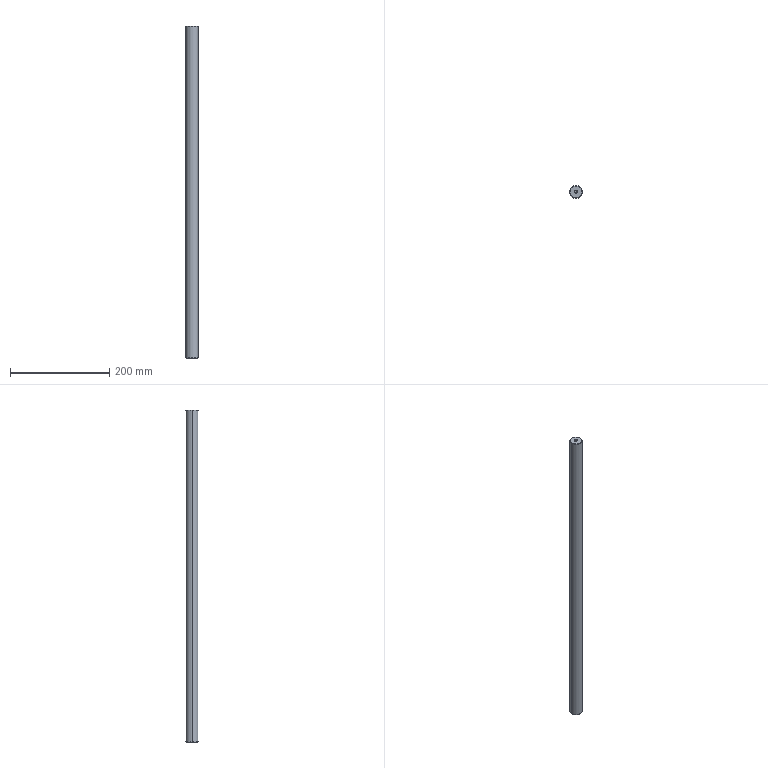Part | STEP file | 1 solid | 20 faces | box 25 x 25 x 670 mm | volume 328039 mm3 | cone 12 | cylinder 6 | plane 2 | commonest cylinder face diameters 5 x4 25 x2
STEP:
#1=CARTESIAN_POINT('',(0.,0.,0.));
#2=DIRECTION('',(0.,0.,1.));
#3=DIRECTION('',(1.,0.,0.));
#4=AXIS2_PLACEMENT_3D('',#1,#2,#3);
#5=CARTESIAN_POINT('',(488.025,0.,665.));
#6=VERTEX_POINT('',#5);
#7=CARTESIAN_POINT('',(481.975,0.,665.));
#8=VERTEX_POINT('',#7);
#9=CARTESIAN_POINT('',(485.,0.,665.));
#10=DIRECTION('',(0.,0.,1.));
#11=DIRECTION('',(1.,0.,0.));
#12=AXIS2_PLACEMENT_3D('',#9,#10,#11);
#13=CIRCLE('',#12,3.025);
#14=CARTESIAN_POINT('',(485.,0.,665.));
#15=DIRECTION('',(0.,0.,1.));
#16=DIRECTION('',(1.,0.,0.));
#17=AXIS2_PLACEMENT_3D('',#14,#15,#16);
#18=CONICAL_SURFACE('',#17,3.025,0.7854);
#19=CARTESIAN_POINT('',(0.,0.));
#20=DIRECTION('',(1.,0.));
#21=VECTOR('',#20,1.);
#22=LINE('',#19,#21);
#23=(GEOMETRIC_REPRESENTATION_CONTEXT(2)PARAMETRIC_REPRESENTATION_CONTEXT()REPRESENTATION_CONTEXT('',''));
#24=DEFINITIONAL_REPRESENTATION('',(#22),#23);
#25=PCURVE('',#18,#24);
#26=CARTESIAN_POINT('',(485.,0.,665.));
#27=DIRECTION('',(0.,0.,1.));
#28=DIRECTION('',(0.,-1.,0.));
#29=AXIS2_PLACEMENT_3D('',#26,#27,#28);
#30=PLANE('',#29);
#31=CARTESIAN_POINT('',(0.,0.));
#32=DIRECTION('',(0.,1.));
#33=AXIS2_PLACEMENT_2D('',#31,#32);
#34=CIRCLE('',#33,3.025);
#35=(GEOMETRIC_REPRESENTATION_CONTEXT(2)PARAMETRIC_REPRESENTATION_CONTEXT()REPRESENTATION_CONTEXT('',''));
#36=DEFINITIONAL_REPRESENTATION('',(#34),#35);
#37=PCURVE('',#30,#36);
#38=SURFACE_CURVE('',#13,(#25,#37),.PCURVE_S1.);
#39=EDGE_CURVE('',#6,#8,#38,.T.);
#40=ORIENTED_EDGE('',*,*,#39,.F.);
#41=CARTESIAN_POINT('',(487.5,0.,664.475));
#42=VERTEX_POINT('',#41);
#43=CARTESIAN_POINT('',(488.025,0.,665.));
#44=DIRECTION('',(0.7071,0.,0.7071));
#45=VECTOR('',#44,1.);
#46=LINE('',#43,#45);
#47=CARTESIAN_POINT('',(0.,0.));
#48=DIRECTION('',(0.,1.));
#49=VECTOR('',#48,1.);
#50=LINE('',#47,#49);
#51=(GEOMETRIC_REPRESENTATION_CONTEXT(2)PARAMETRIC_REPRESENTATION_CONTEXT()REPRESENTATION_CONTEXT('',''));
#52=DEFINITIONAL_REPRESENTATION('',(#50),#51);
#53=PCURVE('',#18,#52);
#54=CARTESIAN_POINT('',(485.,0.,665.));
#55=DIRECTION('',(0.,0.,1.));
#56=DIRECTION('',(1.,0.,0.));
#57=AXIS2_PLACEMENT_3D('',#54,#55,#56);
#58=CONICAL_SURFACE('',#57,3.025,0.7854);
#59=CARTESIAN_POINT('',(6.283,0.));
#60=DIRECTION('',(0.,1.));
#61=VECTOR('',#60,1.);
#62=LINE('',#59,#61);
#63=(GEOMETRIC_REPRESENTATION_CONTEXT(2)PARAMETRIC_REPRESENTATION_CONTEXT()REPRESENTATION_CONTEXT('',''));
#64=DEFINITIONAL_REPRESENTATION('',(#62),#63);
#65=PCURVE('',#58,#64);
#66=SURFACE_CURVE('',#46,(#53,#65),.PCURVE_S1.);
#67=EDGE_CURVE('',#42,#6,#66,.T.);
#68=ORIENTED_EDGE('',*,*,#67,.F.);
#69=CARTESIAN_POINT('',(482.5,0.,664.475));
#70=VERTEX_POINT('',#69);
#71=CARTESIAN_POINT('',(485.,0.,664.475));
#72=DIRECTION('',(0.,0.,1.));
#73=DIRECTION('',(1.,0.,0.));
#74=AXIS2_PLACEMENT_3D('',#71,#72,#73);
#75=CIRCLE('',#74,2.5);
#76=CARTESIAN_POINT('',(0.,-0.525));
#77=DIRECTION('',(1.,0.));
#78=VECTOR('',#77,1.);
#79=LINE('',#76,#78);
#80=(GEOMETRIC_REPRESENTATION_CONTEXT(2)PARAMETRIC_REPRESENTATION_CONTEXT()REPRESENTATION_CONTEXT('',''));
#81=DEFINITIONAL_REPRESENTATION('',(#79),#80);
#82=PCURVE('',#18,#81);
#83=CARTESIAN_POINT('',(485.,0.,665.));
#84=DIRECTION('',(0.,0.,1.));
#85=DIRECTION('',(1.,0.,0.));
#86=AXIS2_PLACEMENT_3D('',#83,#84,#85);
#87=CYLINDRICAL_SURFACE('',#86,2.5);
#88=CARTESIAN_POINT('',(0.,-0.525));
#89=DIRECTION('',(1.,0.));
#90=VECTOR('',#89,1.);
#91=LINE('',#88,#90);
#92=(GEOMETRIC_REPRESENTATION_CONTEXT(2)PARAMETRIC_REPRESENTATION_CONTEXT()REPRESENTATION_CONTEXT('',''));
#93=DEFINITIONAL_REPRESENTATION('',(#91),#92);
#94=PCURVE('',#87,#93);
#95=SURFACE_CURVE('',#75,(#82,#94),.PCURVE_S1.);
#96=EDGE_CURVE('',#42,#70,#95,.T.);
#97=ORIENTED_EDGE('',*,*,#96,.T.);
#98=CARTESIAN_POINT('',(481.975,0.,665.));
#99=DIRECTION('',(-0.7071,0.,0.7071));
#100=VECTOR('',#99,1.);
#101=LINE('',#98,#100);
#102=CARTESIAN_POINT('',(3.142,0.));
#103=DIRECTION('',(0.,1.));
#104=VECTOR('',#103,1.);
#105=LINE('',#102,#104);
#106=(GEOMETRIC_REPRESENTATION_CONTEXT(2)PARAMETRIC_REPRESENTATION_CONTEXT()REPRESENTATION_CONTEXT('',''));
#107=DEFINITIONAL_REPRESENTATION('',(#105),#106);
#108=PCURVE('',#18,#107);
#109=CARTESIAN_POINT('',(3.142,0.));
#110=DIRECTION('',(0.,1.));
#111=VECTOR('',#110,1.);
#112=LINE('',#109,#111);
#113=(GEOMETRIC_REPRESENTATION_CONTEXT(2)PARAMETRIC_REPRESENTATION_CONTEXT()REPRESENTATION_CONTEXT('',''));
#114=DEFINITIONAL_REPRESENTATION('',(#112),#113);
#115=PCURVE('',#58,#114);
#116=SURFACE_CURVE('',#101,(#108,#115),.PCURVE_S1.);
#117=EDGE_CURVE('',#70,#8,#116,.T.);
#118=ORIENTED_EDGE('',*,*,#117,.T.);
#119=EDGE_LOOP('',(#40,#68,#97,#118));
#120=FACE_BOUND('',#119,.F.);
#121=ADVANCED_FACE('',(#120),#18,.F.);
#122=ORIENTED_EDGE('',*,*,#96,.F.);
#123=CARTESIAN_POINT('',(487.5,0.,650.));
#124=VERTEX_POINT('',#123);
#125=CARTESIAN_POINT('',(487.5,0.,665.));
#126=DIRECTION('',(0.,0.,1.));
#127=VECTOR('',#126,1.);
#128=LINE('',#125,#127);
#129=CARTESIAN_POINT('',(0.,0.));
#130=DIRECTION('',(0.,1.));
#131=VECTOR('',#130,1.);
#132=LINE('',#129,#131);
#133=(GEOMETRIC_REPRESENTATION_CONTEXT(2)PARAMETRIC_REPRESENTATION_CONTEXT()REPRESENTATION_CONTEXT('',''));
#134=DEFINITIONAL_REPRESENTATION('',(#132),#133);
#135=PCURVE('',#87,#134);
#136=CARTESIAN_POINT('',(485.,0.,665.));
#137=DIRECTION('',(0.,0.,1.));
#138=DIRECTION('',(1.,0.,0.));
#139=AXIS2_PLACEMENT_3D('',#136,#137,#138);
#140=CYLINDRICAL_SURFACE('',#139,2.5);
#141=CARTESIAN_POINT('',(6.283,0.));
#142=DIRECTION('',(0.,1.));
#143=VECTOR('',#142,1.);
#144=LINE('',#141,#143);
#145=(GEOMETRIC_REPRESENTATION_CONTEXT(2)PARAMETRIC_REPRESENTATION_CONTEXT()REPRESENTATION_CONTEXT('',''));
#146=DEFINITIONAL_REPRESENTATION('',(#144),#145);
#147=PCURVE('',#140,#146);
#148=SURFACE_CURVE('',#128,(#135,#147),.PCURVE_S1.);
#149=EDGE_CURVE('',#124,#42,#148,.T.);
#150=ORIENTED_EDGE('',*,*,#149,.F.);
#151=CARTESIAN_POINT('',(482.5,0.,650.));
#152=VERTEX_POINT('',#151);
#153=CARTESIAN_POINT('',(485.,0.,650.));
#154=DIRECTION('',(0.,0.,1.));
#155=DIRECTION('',(1.,0.,0.));
#156=AXIS2_PLACEMENT_3D('',#153,#154,#155);
#157=CIRCLE('',#156,2.5);
#158=CARTESIAN_POINT('',(0.,-15.));
#159=DIRECTION('',(1.,0.));
#160=VECTOR('',#159,1.);
#161=LINE('',#158,#160);
#162=(GEOMETRIC_REPRESENTATION_CONTEXT(2)PARAMETRIC_REPRESENTATION_CONTEXT()REPRESENTATION_CONTEXT('',''));
#163=DEFINITIONAL_REPRESENTATION('',(#161),#162);
#164=PCURVE('',#87,#163);
#165=CARTESIAN_POINT('',(485.,0.,650.));
#166=DIRECTION('',(0.,0.,1.));
#167=DIRECTION('',(1.,0.,0.));
#168=AXIS2_PLACEMENT_3D('',#165,#166,#167);
#169=CONICAL_SURFACE('',#168,2.5,1.03);
#170=CARTESIAN_POINT('',(0.,0.));
#171=DIRECTION('',(1.,0.));
#172=VECTOR('',#171,1.);
#173=LINE('',#170,#172);
#174=(GEOMETRIC_REPRESENTATION_CONTEXT(2)PARAMETRIC_REPRESENTATION_CONTEXT()REPRESENTATION_CONTEXT('',''));
#175=DEFINITIONAL_REPRESENTATION('',(#173),#174);
#176=PCURVE('',#169,#175);
#177=SURFACE_CURVE('',#157,(#164,#176),.PCURVE_S1.);
#178=EDGE_CURVE('',#124,#152,#177,.T.);
#179=ORIENTED_EDGE('',*,*,#178,.T.);
#180=CARTESIAN_POINT('',(482.5,0.,665.));
#181=DIRECTION('',(0.,0.,1.));
#182=VECTOR('',#181,1.);
#183=LINE('',#180,#182);
#184=CARTESIAN_POINT('',(3.142,0.));
#185=DIRECTION('',(0.,1.));
#186=VECTOR('',#185,1.);
#187=LINE('',#184,#186);
#188=(GEOMETRIC_REPRESENTATION_CONTEXT(2)PARAMETRIC_REPRESENTATION_CONTEXT()REPRESENTATION_CONTEXT('',''));
#189=DEFINITIONAL_REPRESENTATION('',(#187),#188);
#190=PCURVE('',#87,#189);
#191=CARTESIAN_POINT('',(3.142,0.));
#192=DIRECTION('',(0.,1.));
#193=VECTOR('',#192,1.);
#194=LINE('',#191,#193);
#195=(GEOMETRIC_REPRESENTATION_CONTEXT(2)PARAMETRIC_REPRESENTATION_CONTEXT()REPRESENTATION_CONTEXT('',''));
#196=DEFINITIONAL_REPRESENTATION('',(#194),#195);
#197=PCURVE('',#140,#196);
#198=SURFACE_CURVE('',#183,(#190,#197),.PCURVE_S1.);
#199=EDGE_CURVE('',#152,#70,#198,.T.);
#200=ORIENTED_EDGE('',*,*,#199,.T.);
#201=EDGE_LOOP('',(#122,#150,#179,#200));
#202=FACE_BOUND('',#201,.F.);
#203=ADVANCED_FACE('',(#202),#87,.F.);
#204=ORIENTED_EDGE('',*,*,#178,.F.);
#205=CARTESIAN_POINT('',(485.,0.,648.498));
#206=VERTEX_POINT('',#205);
#207=CARTESIAN_POINT('',(487.5,0.,650.));
#208=DIRECTION('',(0.8572,0.,0.515));
#209=VECTOR('',#208,1.);
#210=LINE('',#207,#209);
#211=CARTESIAN_POINT('',(0.,0.));
#212=DIRECTION('',(0.,1.));
#213=VECTOR('',#212,1.);
#214=LINE('',#211,#213);
#215=(GEOMETRIC_REPRESENTATION_CONTEXT(2)PARAMETRIC_REPRESENTATION_CONTEXT()REPRESENTATION_CONTEXT('',''));
#216=DEFINITIONAL_REPRESENTATION('',(#214),#215);
#217=PCURVE('',#169,#216);
#218=CARTESIAN_POINT('',(485.,0.,650.));
#219=DIRECTION('',(0.,0.,1.));
#220=DIRECTION('',(1.,0.,0.));
#221=AXIS2_PLACEMENT_3D('',#218,#219,#220);
#222=CONICAL_SURFACE('',#221,2.5,1.03);
#223=CARTESIAN_POINT('',(6.283,-1.502));
#224=CARTESIAN_POINT('',(6.283,-1.479));
#225=CARTESIAN_POINT('',(6.283,-1.434));
#226=CARTESIAN_POINT('',(6.283,-1.366));
#227=CARTESIAN_POINT('',(6.283,-1.297));
#228=CARTESIAN_POINT('',(6.283,-1.229));
#229=CARTESIAN_POINT('',(6.283,-1.161));
#230=CARTESIAN_POINT('',(6.283,-1.092));
#231=CARTESIAN_POINT('',(6.283,-1.024));
#232=CARTESIAN_POINT('',(6.283,-0.9559));
#233=CARTESIAN_POINT('',(6.283,-0.8876));
#234=CARTESIAN_POINT('',(6.283,-0.8194));
#235=CARTESIAN_POINT('',(6.283,-0.7511));
#236=CARTESIAN_POINT('',(6.283,-0.6828));
#237=CARTESIAN_POINT('',(6.283,-0.6145));
#238=CARTESIAN_POINT('',(6.283,-0.5462));
#239=CARTESIAN_POINT('',(6.283,-0.478));
#240=CARTESIAN_POINT('',(6.283,-0.4097));
#241=CARTESIAN_POINT('',(6.283,-0.3414));
#242=CARTESIAN_POINT('',(6.283,-0.2731));
#243=CARTESIAN_POINT('',(6.283,-0.2048));
#244=CARTESIAN_POINT('',(6.283,-0.1366));
#245=CARTESIAN_POINT('',(6.283,-0.06828));
#246=CARTESIAN_POINT('',(6.283,-0.02276));
#247=CARTESIAN_POINT('',(6.283,0.));
#248=B_SPLINE_CURVE_WITH_KNOTS('',3,(#223,#224,#225,#226,#227,#228,#229,#230,#231,#232,#233,#234,#235,#236,#237,#238,#239,#240,#241,#242,#243,#244,#245,#246,#247),.UNSPECIFIED.,.F.,.F.,(4,1,1,1,1,1,1,1,1,1,1,1,1,1,1,1,1,1,1,1,1,1,4),(-2.917,-2.784,-2.651,-2.519,-2.386,-2.254,-2.121,-1.989,-1.856,-1.723,-1.591,-1.458,-1.326,-1.193,-1.061,-0.928,-0.7954,-0.6629,-0.5303,-0.3977,-0.2651,-0.1326,0.),.UNSPECIFIED.);
#249=(GEOMETRIC_REPRESENTATION_CONTEXT(2)PARAMETRIC_REPRESENTATION_CONTEXT()REPRESENTATION_CONTEXT('',''));
#250=DEFINITIONAL_REPRESENTATION('',(#248),#249);
#251=PCURVE('',#222,#250);
#252=SURFACE_CURVE('',#210,(#217,#251),.PCURVE_S1.);
#253=EDGE_CURVE('',#206,#124,#252,.T.);
#254=ORIENTED_EDGE('',*,*,#253,.F.);
#255=CARTESIAN_POINT('',(482.5,0.,650.));
#256=DIRECTION('',(-0.8572,0.,0.515));
#257=VECTOR('',#256,1.);
#258=LINE('',#255,#257);
#259=CARTESIAN_POINT('',(3.142,0.));
#260=DIRECTION('',(0.,1.));
#261=VECTOR('',#260,1.);
#262=LINE('',#259,#261);
#263=(GEOMETRIC_REPRESENTATION_CONTEXT(2)PARAMETRIC_REPRESENTATION_CONTEXT()REPRESENTATION_CONTEXT('',''));
#264=DEFINITIONAL_REPRESENTATION('',(#262),#263);
#265=PCURVE('',#169,#264);
#266=CARTESIAN_POINT('',(3.142,0.));
#267=DIRECTION('',(0.,1.));
#268=VECTOR('',#267,1.);
#269=LINE('',#266,#268);
#270=(GEOMETRIC_REPRESENTATION_CONTEXT(2)PARAMETRIC_REPRESENTATION_CONTEXT()REPRESENTATION_CONTEXT('',''));
#271=DEFINITIONAL_REPRESENTATION('',(#269),#270);
#272=PCURVE('',#222,#271);
#273=SURFACE_CURVE('',#258,(#265,#272),.PCURVE_S1.);
#274=EDGE_CURVE('',#206,#152,#273,.T.);
#275=ORIENTED_EDGE('',*,*,#274,.T.);
#276=EDGE_LOOP('',(#204,#254,#275));
#277=FACE_BOUND('',#276,.F.);
#278=ADVANCED_FACE('',(#277),#169,.F.);
#279=CARTESIAN_POINT('',(473.5,0.,-5.));
#280=VERTEX_POINT('',#279);
#281=CARTESIAN_POINT('',(472.5,0.,-4.));
#282=VERTEX_POINT('',#281);
#283=CARTESIAN_POINT('',(472.5,0.,-4.));
#284=DIRECTION('',(-0.7071,0.,0.7071));
#285=VECTOR('',#284,1.);
#286=LINE('',#283,#285);
#287=CARTESIAN_POINT('',(485.,0.,-4.));
#288=DIRECTION('',(0.,0.,1.));
#289=DIRECTION('',(1.,0.,0.));
#290=AXIS2_PLACEMENT_3D('',#287,#288,#289);
#291=CONICAL_SURFACE('',#290,12.5,0.7854);
#292=CARTESIAN_POINT('',(3.142,0.));
#293=DIRECTION('',(0.,1.));
#294=VECTOR('',#293,1.);
#295=LINE('',#292,#294);
#296=(GEOMETRIC_REPRESENTATION_CONTEXT(2)PARAMETRIC_REPRESENTATION_CONTEXT()REPRESENTATION_CONTEXT('',''));
#297=DEFINITIONAL_REPRESENTATION('',(#295),#296);
#298=PCURVE('',#291,#297);
#299=CARTESIAN_POINT('',(485.,0.,-4.));
#300=DIRECTION('',(0.,0.,1.));
#301=DIRECTION('',(1.,0.,0.));
#302=AXIS2_PLACEMENT_3D('',#299,#300,#301);
#303=CONICAL_SURFACE('',#302,12.5,0.7854);
#304=CARTESIAN_POINT('',(3.142,0.));
#305=DIRECTION('',(0.,1.));
#306=VECTOR('',#305,1.);
#307=LINE('',#304,#306);
#308=(GEOMETRIC_REPRESENTATION_CONTEXT(2)PARAMETRIC_REPRESENTATION_CONTEXT()REPRESENTATION_CONTEXT('',''));
#309=DEFINITIONAL_REPRESENTATION('',(#307),#308);
#310=PCURVE('',#303,#309);
#311=SURFACE_CURVE('',#286,(#298,#310),.PCURVE_S1.);
#312=EDGE_CURVE('',#280,#282,#311,.T.);
#313=ORIENTED_EDGE('',*,*,#312,.F.);
#314=CARTESIAN_POINT('',(496.5,0.,-5.));
#315=VERTEX_POINT('',#314);
#316=CARTESIAN_POINT('',(485.,0.,-5.));
#317=DIRECTION('',(0.,0.,-1.));
#318=DIRECTION('',(1.,0.,0.));
#319=AXIS2_PLACEMENT_3D('',#316,#317,#318);
#320=CIRCLE('',#319,11.5);
#321=CARTESIAN_POINT('',(6.283,-1.));
#322=DIRECTION('',(-1.,0.));
#323=VECTOR('',#322,1.);
#324=LINE('',#321,#323);
#325=(GEOMETRIC_REPRESENTATION_CONTEXT(2)PARAMETRIC_REPRESENTATION_CONTEXT()REPRESENTATION_CONTEXT('',''));
#326=DEFINITIONAL_REPRESENTATION('',(#324),#325);
#327=PCURVE('',#291,#326);
#328=CARTESIAN_POINT('',(485.,0.,-5.));
#329=DIRECTION('',(0.,0.,1.));
#330=DIRECTION('',(0.,-1.,0.));
#331=AXIS2_PLACEMENT_3D('',#328,#329,#330);
#332=PLANE('',#331);
#333=CARTESIAN_POINT('',(0.,11.5));
#334=CARTESIAN_POINT('',(19.919,11.5));
#335=CARTESIAN_POINT('',(9.959,-5.75));
#336=CARTESIAN_POINT('',(0.,-23.));
#337=CARTESIAN_POINT('',(-9.959,-5.75));
#338=CARTESIAN_POINT('',(-19.919,11.5));
#339=CARTESIAN_POINT('',(0.,11.5));
#340=(BOUNDED_CURVE()B_SPLINE_CURVE(2,(#333,#334,#335,#336,#337,#338,#339),.UNSPECIFIED.,.T.,.F.)B_SPLINE_CURVE_WITH_KNOTS((1,2,2,2,2,1),(-2.094,0.,2.094,4.189,6.283,8.378),.UNSPECIFIED.)CURVE()GEOMETRIC_REPRESENTATION_ITEM()RATIONAL_B_SPLINE_CURVE((1.,0.5,1.,0.5,1.,0.5,1.))REPRESENTATION_ITEM(''));
#341=(GEOMETRIC_REPRESENTATION_CONTEXT(2)PARAMETRIC_REPRESENTATION_CONTEXT()REPRESENTATION_CONTEXT('',''));
#342=DEFINITIONAL_REPRESENTATION('',(#340),#341);
#343=PCURVE('',#332,#342);
#344=SURFACE_CURVE('',#320,(#327,#343),.PCURVE_S1.);
#345=EDGE_CURVE('',#315,#280,#344,.T.);
#346=ORIENTED_EDGE('',*,*,#345,.F.);
#347=CARTESIAN_POINT('',(497.5,0.,-4.));
#348=VERTEX_POINT('',#347);
#349=CARTESIAN_POINT('',(497.5,0.,-4.));
#350=DIRECTION('',(0.7071,0.,0.7071));
#351=VECTOR('',#350,1.);
#352=LINE('',#349,#351);
#353=CARTESIAN_POINT('',(6.283,0.));
#354=DIRECTION('',(0.,1.));
#355=VECTOR('',#354,1.);
#356=LINE('',#353,#355);
#357=(GEOMETRIC_REPRESENTATION_CONTEXT(2)PARAMETRIC_REPRESENTATION_CONTEXT()REPRESENTATION_CONTEXT('',''));
#358=DEFINITIONAL_REPRESENTATION('',(#356),#357);
#359=PCURVE('',#291,#358);
#360=CARTESIAN_POINT('',(0.,0.));
#361=DIRECTION('',(0.,1.));
#362=VECTOR('',#361,1.);
#363=LINE('',#360,#362);
#364=(GEOMETRIC_REPRESENTATION_CONTEXT(2)PARAMETRIC_REPRESENTATION_CONTEXT()REPRESENTATION_CONTEXT('',''));
#365=DEFINITIONAL_REPRESENTATION('',(#363),#364);
#366=PCURVE('',#303,#365);
#367=SURFACE_CURVE('',#352,(#359,#366),.PCURVE_S1.);
#368=EDGE_CURVE('',#315,#348,#367,.T.);
#369=ORIENTED_EDGE('',*,*,#368,.T.);
#370=CARTESIAN_POINT('',(485.,0.,-4.));
#371=DIRECTION('',(0.,0.,1.));
#372=DIRECTION('',(1.,0.,0.));
#373=AXIS2_PLACEMENT_3D('',#370,#371,#372);
#374=CIRCLE('',#373,12.5);
#375=CARTESIAN_POINT('',(0.,0.));
#376=DIRECTION('',(1.,0.));
#377=VECTOR('',#376,1.);
#378=LINE('',#375,#377);
#379=(GEOMETRIC_REPRESENTATION_CONTEXT(2)PARAMETRIC_REPRESENTATION_CONTEXT()REPRESENTATION_CONTEXT('',''));
#380=DEFINITIONAL_REPRESENTATION('',(#378),#379);
#381=PCURVE('',#291,#380);
#382=CARTESIAN_POINT('',(485.,0.,-5.));
#383=DIRECTION('',(0.,0.,1.));
#384=DIRECTION('',(1.,0.,0.));
#385=AXIS2_PLACEMENT_3D('',#382,#383,#384);
#386=CYLINDRICAL_SURFACE('',#385,12.5);
#387=CARTESIAN_POINT('',(0.,1.));
#388=DIRECTION('',(1.,0.));
#389=VECTOR('',#388,1.);
#390=LINE('',#387,#389);
#391=(GEOMETRIC_REPRESENTATION_CONTEXT(2)PARAMETRIC_REPRESENTATION_CONTEXT()REPRESENTATION_CONTEXT('',''));
#392=DEFINITIONAL_REPRESENTATION('',(#390),#391);
#393=PCURVE('',#386,#392);
#394=SURFACE_CURVE('',#374,(#381,#393),.PCURVE_S1.);
#395=EDGE_CURVE('',#282,#348,#394,.T.);
#396=ORIENTED_EDGE('',*,*,#395,.F.);
#397=EDGE_LOOP('',(#313,#346,#369,#396));
#398=FACE_BOUND('',#397,.T.);
#399=ADVANCED_FACE('',(#398),#291,.T.);
#400=CARTESIAN_POINT('',(496.5,0.,665.));
#401=VERTEX_POINT('',#400);
#402=CARTESIAN_POINT('',(497.5,0.,664.));
#403=VERTEX_POINT('',#402);
#404=CARTESIAN_POINT('',(496.5,0.,665.));
#405=DIRECTION('',(0.7071,0.,-0.7071));
#406=VECTOR('',#405,1.);
#407=LINE('',#404,#406);
#408=CARTESIAN_POINT('',(485.,0.,665.));
#409=DIRECTION('',(0.,0.,-1.));
#410=DIRECTION('',(-1.,0.,0.));
#411=AXIS2_PLACEMENT_3D('',#408,#409,#410);
#412=CONICAL_SURFACE('',#411,11.5,0.7854);
#413=CARTESIAN_POINT('',(3.142,0.));
#414=DIRECTION('',(0.,1.));
#415=VECTOR('',#414,1.);
#416=LINE('',#413,#415);
#417=(GEOMETRIC_REPRESENTATION_CONTEXT(2)PARAMETRIC_REPRESENTATION_CONTEXT()REPRESENTATION_CONTEXT('',''));
#418=DEFINITIONAL_REPRESENTATION('',(#416),#417);
#419=PCURVE('',#412,#418);
#420=CARTESIAN_POINT('',(485.,0.,665.));
#421=DIRECTION('',(0.,0.,-1.));
#422=DIRECTION('',(-1.,0.,0.));
#423=AXIS2_PLACEMENT_3D('',#420,#421,#422);
#424=CONICAL_SURFACE('',#423,11.5,0.7854);
#425=CARTESIAN_POINT('',(3.142,0.));
#426=DIRECTION('',(0.,1.));
#427=VECTOR('',#426,1.);
#428=LINE('',#425,#427);
#429=(GEOMETRIC_REPRESENTATION_CONTEXT(2)PARAMETRIC_REPRESENTATION_CONTEXT()REPRESENTATION_CONTEXT('',''));
#430=DEFINITIONAL_REPRESENTATION('',(#428),#429);
#431=PCURVE('',#424,#430);
#432=SURFACE_CURVE('',#407,(#419,#431),.PCURVE_S1.);
#433=EDGE_CURVE('',#401,#403,#432,.T.);
#434=ORIENTED_EDGE('',*,*,#433,.F.);
#435=CARTESIAN_POINT('',(473.5,0.,665.));
#436=VERTEX_POINT('',#435);
#437=CARTESIAN_POINT('',(485.,0.,665.));
#438=DIRECTION('',(0.,0.,1.));
#439=DIRECTION('',(1.,0.,0.));
#440=AXIS2_PLACEMENT_3D('',#437,#438,#439);
#441=CIRCLE('',#440,11.5);
#442=CARTESIAN_POINT('',(9.425,0.));
#443=DIRECTION('',(-1.,0.));
#444=VECTOR('',#443,1.);
#445=LINE('',#442,#444);
#446=(GEOMETRIC_REPRESENTATION_CONTEXT(2)PARAMETRIC_REPRESENTATION_CONTEXT()REPRESENTATION_CONTEXT('',''));
#447=DEFINITIONAL_REPRESENTATION('',(#445),#446);
#448=PCURVE('',#412,#447);
#449=CARTESIAN_POINT('',(0.,0.));
#450=DIRECTION('',(0.,1.));
#451=AXIS2_PLACEMENT_2D('',#449,#450);
#452=CIRCLE('',#451,11.5);
#453=(GEOMETRIC_REPRESENTATION_CONTEXT(2)PARAMETRIC_REPRESENTATION_CONTEXT()REPRESENTATION_CONTEXT('',''));
#454=DEFINITIONAL_REPRESENTATION('',(#452),#453);
#455=PCURVE('',#30,#454);
#456=SURFACE_CURVE('',#441,(#448,#455),.PCURVE_S1.);
#457=EDGE_CURVE('',#436,#401,#456,.T.);
#458=ORIENTED_EDGE('',*,*,#457,.F.);
#459=CARTESIAN_POINT('',(472.5,0.,664.));
#460=VERTEX_POINT('',#459);
#461=CARTESIAN_POINT('',(473.5,0.,665.));
#462=DIRECTION('',(-0.7071,0.,-0.7071));
#463=VECTOR('',#462,1.);
#464=LINE('',#461,#463);
#465=CARTESIAN_POINT('',(6.283,0.));
#466=DIRECTION('',(0.,1.));
#467=VECTOR('',#466,1.);
#468=LINE('',#465,#467);
#469=(GEOMETRIC_REPRESENTATION_CONTEXT(2)PARAMETRIC_REPRESENTATION_CONTEXT()REPRESENTATION_CONTEXT('',''));
#470=DEFINITIONAL_REPRESENTATION('',(#468),#469);
#471=PCURVE('',#412,#470);
#472=CARTESIAN_POINT('',(0.,0.));
#473=DIRECTION('',(0.,1.));
#474=VECTOR('',#473,1.);
#475=LINE('',#472,#474);
#476=(GEOMETRIC_REPRESENTATION_CONTEXT(2)PARAMETRIC_REPRESENTATION_CONTEXT()REPRESENTATION_CONTEXT('',''));
#477=DEFINITIONAL_REPRESENTATION('',(#475),#476);
#478=PCURVE('',#424,#477);
#479=SURFACE_CURVE('',#464,(#471,#478),.PCURVE_S1.);
#480=EDGE_CURVE('',#436,#460,#479,.T.);
#481=ORIENTED_EDGE('',*,*,#480,.T.);
#482=CARTESIAN_POINT('',(485.,0.,664.));
#483=DIRECTION('',(0.,0.,-1.));
#484=DIRECTION('',(1.,0.,0.));
#485=AXIS2_PLACEMENT_3D('',#482,#483,#484);
#486=CIRCLE('',#485,12.5);
#487=CARTESIAN_POINT('',(3.142,1.));
#488=DIRECTION('',(1.,0.));
#489=VECTOR('',#488,1.);
#490=LINE('',#487,#489);
#491=(GEOMETRIC_REPRESENTATION_CONTEXT(2)PARAMETRIC_REPRESENTATION_CONTEXT()REPRESENTATION_CONTEXT('',''));
#492=DEFINITIONAL_REPRESENTATION('',(#490),#491);
#493=PCURVE('',#412,#492);
#494=CARTESIAN_POINT('',(6.283,669.));
#495=DIRECTION('',(-1.,0.));
#496=VECTOR('',#495,1.);
#497=LINE('',#494,#496);
#498=(GEOMETRIC_REPRESENTATION_CONTEXT(2)PARAMETRIC_REPRESENTATION_CONTEXT()REPRESENTATION_CONTEXT('',''));
#499=DEFINITIONAL_REPRESENTATION('',(#497),#498);
#500=PCURVE('',#386,#499);
#501=SURFACE_CURVE('',#486,(#493,#500),.PCURVE_S1.);
#502=EDGE_CURVE('',#403,#460,#501,.T.);
#503=ORIENTED_EDGE('',*,*,#502,.F.);
#504=EDGE_LOOP('',(#434,#458,#481,#503));
#505=FACE_BOUND('',#504,.T.);
#506=ADVANCED_FACE('',(#505),#412,.T.);
#507=CARTESIAN_POINT('',(481.975,0.,-5.));
#508=VERTEX_POINT('',#507);
#509=CARTESIAN_POINT('',(488.025,0.,-5.));
#510=VERTEX_POINT('',#509);
#511=CARTESIAN_POINT('',(485.,0.,-5.));
#512=DIRECTION('',(0.,0.,-1.));
#513=DIRECTION('',(-1.,0.,0.));
#514=AXIS2_PLACEMENT_3D('',#511,#512,#513);
#515=CIRCLE('',#514,3.025);
#516=CARTESIAN_POINT('',(485.,0.,-5.));
#517=DIRECTION('',(0.,0.,-1.));
#518=DIRECTION('',(-1.,0.,0.));
#519=AXIS2_PLACEMENT_3D('',#516,#517,#518);
#520=CONICAL_SURFACE('',#519,3.025,0.7854);
#521=CARTESIAN_POINT('',(0.,0.));
#522=DIRECTION('',(1.,0.));
#523=VECTOR('',#522,1.);
#524=LINE('',#521,#523);
#525=(GEOMETRIC_REPRESENTATION_CONTEXT(2)PARAMETRIC_REPRESENTATION_CONTEXT()REPRESENTATION_CONTEXT('',''));
#526=DEFINITIONAL_REPRESENTATION('',(#524),#525);
#527=PCURVE('',#520,#526);
#528=CARTESIAN_POINT('',(0.,-3.025));
#529=CARTESIAN_POINT('',(-5.239,-3.025));
#530=CARTESIAN_POINT('',(-2.62,1.512));
#531=CARTESIAN_POINT('',(0.,6.05));
#532=CARTESIAN_POINT('',(2.62,1.512));
#533=CARTESIAN_POINT('',(5.239,-3.025));
#534=CARTESIAN_POINT('',(0.,-3.025));
#535=(BOUNDED_CURVE()B_SPLINE_CURVE(2,(#528,#529,#530,#531,#532,#533,#534),.UNSPECIFIED.,.T.,.F.)B_SPLINE_CURVE_WITH_KNOTS((1,2,2,2,2,1),(-2.094,0.,2.094,4.189,6.283,8.378),.UNSPECIFIED.)CURVE()GEOMETRIC_REPRESENTATION_ITEM()RATIONAL_B_SPLINE_CURVE((1.,0.5,1.,0.5,1.,0.5,1.))REPRESENTATION_ITEM(''));
#536=(GEOMETRIC_REPRESENTATION_CONTEXT(2)PARAMETRIC_REPRESENTATION_CONTEXT()REPRESENTATION_CONTEXT('',''));
#537=DEFINITIONAL_REPRESENTATION('',(#535),#536);
#538=PCURVE('',#332,#537);
#539=SURFACE_CURVE('',#515,(#527,#538),.PCURVE_S1.);
#540=EDGE_CURVE('',#508,#510,#539,.T.);
#541=ORIENTED_EDGE('',*,*,#540,.F.);
#542=CARTESIAN_POINT('',(482.5,0.,-4.475));
#543=VERTEX_POINT('',#542);
#544=CARTESIAN_POINT('',(481.975,0.,-5.));
#545=DIRECTION('',(-0.7071,0.,-0.7071));
#546=VECTOR('',#545,1.);
#547=LINE('',#544,#546);
#548=CARTESIAN_POINT('',(0.,0.));
#549=DIRECTION('',(0.,1.));
#550=VECTOR('',#549,1.);
#551=LINE('',#548,#550);
#552=(GEOMETRIC_REPRESENTATION_CONTEXT(2)PARAMETRIC_REPRESENTATION_CONTEXT()REPRESENTATION_CONTEXT('',''));
#553=DEFINITIONAL_REPRESENTATION('',(#551),#552);
#554=PCURVE('',#520,#553);
#555=CARTESIAN_POINT('',(485.,0.,-5.));
#556=DIRECTION('',(0.,0.,-1.));
#557=DIRECTION('',(-1.,0.,0.));
#558=AXIS2_PLACEMENT_3D('',#555,#556,#557);
#559=CONICAL_SURFACE('',#558,3.025,0.7854);
#560=CARTESIAN_POINT('',(6.283,0.));
#561=DIRECTION('',(0.,1.));
#562=VECTOR('',#561,1.);
#563=LINE('',#560,#562);
#564=(GEOMETRIC_REPRESENTATION_CONTEXT(2)PARAMETRIC_REPRESENTATION_CONTEXT()REPRESENTATION_CONTEXT('',''));
#565=DEFINITIONAL_REPRESENTATION('',(#563),#564);
#566=PCURVE('',#559,#565);
#567=SURFACE_CURVE('',#547,(#554,#566),.PCURVE_S1.);
#568=EDGE_CURVE('',#543,#508,#567,.T.);
#569=ORIENTED_EDGE('',*,*,#568,.F.);
#570=CARTESIAN_POINT('',(487.5,0.,-4.475));
#571=VERTEX_POINT('',#570);
#572=CARTESIAN_POINT('',(485.,0.,-4.475));
#573=DIRECTION('',(0.,0.,-1.));
#574=DIRECTION('',(-1.,0.,0.));
#575=AXIS2_PLACEMENT_3D('',#572,#573,#574);
#576=CIRCLE('',#575,2.5);
#577=CARTESIAN_POINT('',(0.,-0.525));
#578=DIRECTION('',(1.,0.));
#579=VECTOR('',#578,1.);
#580=LINE('',#577,#579);
#581=(GEOMETRIC_REPRESENTATION_CONTEXT(2)PARAMETRIC_REPRESENTATION_CONTEXT()REPRESENTATION_CONTEXT('',''));
#582=DEFINITIONAL_REPRESENTATION('',(#580),#581);
#583=PCURVE('',#520,#582);
#584=CARTESIAN_POINT('',(485.,0.,-5.));
#585=DIRECTION('',(0.,0.,-1.));
#586=DIRECTION('',(-1.,0.,0.));
#587=AXIS2_PLACEMENT_3D('',#584,#585,#586);
#588=CYLINDRICAL_SURFACE('',#587,2.5);
#589=CARTESIAN_POINT('',(0.,-0.525));
#590=DIRECTION('',(1.,0.));
#591=VECTOR('',#590,1.);
#592=LINE('',#589,#591);
#593=(GEOMETRIC_REPRESENTATION_CONTEXT(2)PARAMETRIC_REPRESENTATION_CONTEXT()REPRESENTATION_CONTEXT('',''));
#594=DEFINITIONAL_REPRESENTATION('',(#592),#593);
#595=PCURVE('',#588,#594);
#596=SURFACE_CURVE('',#576,(#583,#595),.PCURVE_S1.);
#597=EDGE_CURVE('',#543,#571,#596,.T.);
#598=ORIENTED_EDGE('',*,*,#597,.T.);
#599=CARTESIAN_POINT('',(488.025,0.,-5.));
#600=DIRECTION('',(0.7071,0.,-0.7071));
#601=VECTOR('',#600,1.);
#602=LINE('',#599,#601);
#603=CARTESIAN_POINT('',(3.142,0.));
#604=DIRECTION('',(0.,1.));
#605=VECTOR('',#604,1.);
#606=LINE('',#603,#605);
#607=(GEOMETRIC_REPRESENTATION_CONTEXT(2)PARAMETRIC_REPRESENTATION_CONTEXT()REPRESENTATION_CONTEXT('',''));
#608=DEFINITIONAL_REPRESENTATION('',(#606),#607);
#609=PCURVE('',#520,#608);
#610=CARTESIAN_POINT('',(3.142,0.));
#611=DIRECTION('',(0.,1.));
#612=VECTOR('',#611,1.);
#613=LINE('',#610,#612);
#614=(GEOMETRIC_REPRESENTATION_CONTEXT(2)PARAMETRIC_REPRESENTATION_CONTEXT()REPRESENTATION_CONTEXT('',''));
#615=DEFINITIONAL_REPRESENTATION('',(#613),#614);
#616=PCURVE('',#559,#615);
#617=SURFACE_CURVE('',#602,(#609,#616),.PCURVE_S1.);
#618=EDGE_CURVE('',#571,#510,#617,.T.);
#619=ORIENTED_EDGE('',*,*,#618,.T.);
#620=EDGE_LOOP('',(#541,#569,#598,#619));
#621=FACE_BOUND('',#620,.F.);
#622=ADVANCED_FACE('',(#621),#520,.F.);
#623=ORIENTED_EDGE('',*,*,#597,.F.);
#624=CARTESIAN_POINT('',(482.5,0.,18.));
#625=VERTEX_POINT('',#624);
#626=CARTESIAN_POINT('',(482.5,0.,-5.));
#627=DIRECTION('',(0.,0.,-1.));
#628=VECTOR('',#627,1.);
#629=LINE('',#626,#628);
#630=CARTESIAN_POINT('',(0.,0.));
#631=DIRECTION('',(0.,1.));
#632=VECTOR('',#631,1.);
#633=LINE('',#630,#632);
#634=(GEOMETRIC_REPRESENTATION_CONTEXT(2)PARAMETRIC_REPRESENTATION_CONTEXT()REPRESENTATION_CONTEXT('',''));
#635=DEFINITIONAL_REPRESENTATION('',(#633),#634);
#636=PCURVE('',#588,#635);
#637=CARTESIAN_POINT('',(485.,0.,-5.));
#638=DIRECTION('',(0.,0.,-1.));
#639=DIRECTION('',(-1.,0.,0.));
#640=AXIS2_PLACEMENT_3D('',#637,#638,#639);
#641=CYLINDRICAL_SURFACE('',#640,2.5);
#642=CARTESIAN_POINT('',(6.283,0.));
#643=DIRECTION('',(0.,1.));
#644=VECTOR('',#643,1.);
#645=LINE('',#642,#644);
#646=(GEOMETRIC_REPRESENTATION_CONTEXT(2)PARAMETRIC_REPRESENTATION_CONTEXT()REPRESENTATION_CONTEXT('',''));
#647=DEFINITIONAL_REPRESENTATION('',(#645),#646);
#648=PCURVE('',#641,#647);
#649=SURFACE_CURVE('',#629,(#636,#648),.PCURVE_S1.);
#650=EDGE_CURVE('',#625,#543,#649,.T.);
#651=ORIENTED_EDGE('',*,*,#650,.F.);
#652=CARTESIAN_POINT('',(487.5,0.,18.));
#653=VERTEX_POINT('',#652);
#654=CARTESIAN_POINT('',(485.,0.,18.));
#655=DIRECTION('',(0.,0.,-1.));
#656=DIRECTION('',(-1.,0.,0.));
#657=AXIS2_PLACEMENT_3D('',#654,#655,#656);
#658=CIRCLE('',#657,2.5);
#659=CARTESIAN_POINT('',(0.,-23.));
#660=DIRECTION('',(1.,0.));
#661=VECTOR('',#660,1.);
#662=LINE('',#659,#661);
#663=(GEOMETRIC_REPRESENTATION_CONTEXT(2)PARAMETRIC_REPRESENTATION_CONTEXT()REPRESENTATION_CONTEXT('',''));
#664=DEFINITIONAL_REPRESENTATION('',(#662),#663);
#665=PCURVE('',#588,#664);
#666=CARTESIAN_POINT('',(485.,0.,18.));
#667=DIRECTION('',(0.,0.,-1.));
#668=DIRECTION('',(-1.,0.,0.));
#669=AXIS2_PLACEMENT_3D('',#666,#667,#668);
#670=CONICAL_SURFACE('',#669,2.5,1.03);
#671=CARTESIAN_POINT('',(0.,0.));
#672=DIRECTION('',(1.,0.));
#673=VECTOR('',#672,1.);
#674=LINE('',#671,#673);
#675=(GEOMETRIC_REPRESENTATION_CONTEXT(2)PARAMETRIC_REPRESENTATION_CONTEXT()REPRESENTATION_CONTEXT('',''));
#676=DEFINITIONAL_REPRESENTATION('',(#674),#675);
#677=PCURVE('',#670,#676);
#678=SURFACE_CURVE('',#658,(#665,#677),.PCURVE_S1.);
#679=EDGE_CURVE('',#625,#653,#678,.T.);
#680=ORIENTED_EDGE('',*,*,#679,.T.);
#681=CARTESIAN_POINT('',(487.5,0.,-5.));
#682=DIRECTION('',(0.,0.,-1.));
#683=VECTOR('',#682,1.);
#684=LINE('',#681,#683);
#685=CARTESIAN_POINT('',(3.142,0.));
#686=DIRECTION('',(0.,1.));
#687=VECTOR('',#686,1.);
#688=LINE('',#685,#687);
#689=(GEOMETRIC_REPRESENTATION_CONTEXT(2)PARAMETRIC_REPRESENTATION_CONTEXT()REPRESENTATION_CONTEXT('',''));
#690=DEFINITIONAL_REPRESENTATION('',(#688),#689);
#691=PCURVE('',#588,#690);
#692=CARTESIAN_POINT('',(3.142,0.));
#693=DIRECTION('',(0.,1.));
#694=VECTOR('',#693,1.);
#695=LINE('',#692,#694);
#696=(GEOMETRIC_REPRESENTATION_CONTEXT(2)PARAMETRIC_REPRESENTATION_CONTEXT()REPRESENTATION_CONTEXT('',''));
#697=DEFINITIONAL_REPRESENTATION('',(#695),#696);
#698=PCURVE('',#641,#697);
#699=SURFACE_CURVE('',#684,(#691,#698),.PCURVE_S1.);
#700=EDGE_CURVE('',#653,#571,#699,.T.);
#701=ORIENTED_EDGE('',*,*,#700,.T.);
#702=EDGE_LOOP('',(#623,#651,#680,#701));
#703=FACE_BOUND('',#702,.F.);
#704=ADVANCED_FACE('',(#703),#588,.F.);
#705=ORIENTED_EDGE('',*,*,#679,.F.);
#706=CARTESIAN_POINT('',(485.,0.,19.502));
#707=VERTEX_POINT('',#706);
#708=CARTESIAN_POINT('',(482.5,0.,18.));
#709=DIRECTION('',(-0.8572,0.,-0.515));
#710=VECTOR('',#709,1.);
#711=LINE('',#708,#710);
#712=CARTESIAN_POINT('',(0.,-1.502));
#713=CARTESIAN_POINT('',(0.,-1.479));
#714=CARTESIAN_POINT('',(0.,-1.434));
#715=CARTESIAN_POINT('',(0.,-1.366));
#716=CARTESIAN_POINT('',(0.,-1.297));
#717=CARTESIAN_POINT('',(0.,-1.229));
#718=CARTESIAN_POINT('',(0.,-1.161));
#719=CARTESIAN_POINT('',(0.,-1.092));
#720=CARTESIAN_POINT('',(0.,-1.024));
#721=CARTESIAN_POINT('',(0.,-0.9559));
#722=CARTESIAN_POINT('',(0.,-0.8876));
#723=CARTESIAN_POINT('',(0.,-0.8194));
#724=CARTESIAN_POINT('',(0.,-0.7511));
#725=CARTESIAN_POINT('',(0.,-0.6828));
#726=CARTESIAN_POINT('',(0.,-0.6145));
#727=CARTESIAN_POINT('',(0.,-0.5462));
#728=CARTESIAN_POINT('',(0.,-0.478));
#729=CARTESIAN_POINT('',(0.,-0.4097));
#730=CARTESIAN_POINT('',(0.,-0.3414));
#731=CARTESIAN_POINT('',(0.,-0.2731));
#732=CARTESIAN_POINT('',(0.,-0.2048));
#733=CARTESIAN_POINT('',(0.,-0.1366));
#734=CARTESIAN_POINT('',(0.,-0.06828));
#735=CARTESIAN_POINT('',(0.,-0.02276));
#736=CARTESIAN_POINT('',(0.,0.));
#737=B_SPLINE_CURVE_WITH_KNOTS('',3,(#712,#713,#714,#715,#716,#717,#718,#719,#720,#721,#722,#723,#724,#725,#726,#727,#728,#729,#730,#731,#732,#733,#734,#735,#736),.UNSPECIFIED.,.F.,.F.,(4,1,1,1,1,1,1,1,1,1,1,1,1,1,1,1,1,1,1,1,1,1,4),(-2.917,-2.784,-2.651,-2.519,-2.386,-2.254,-2.121,-1.989,-1.856,-1.723,-1.591,-1.458,-1.326,-1.193,-1.061,-0.928,-0.7954,-0.6629,-0.5303,-0.3977,-0.2651,-0.1326,0.),.QUASI_UNIFORM_KNOTS.);
#738=(GEOMETRIC_REPRESENTATION_CONTEXT(2)PARAMETRIC_REPRESENTATION_CONTEXT()REPRESENTATION_CONTEXT('',''));
#739=DEFINITIONAL_REPRESENTATION('',(#737),#738);
#740=PCURVE('',#670,#739);
#741=CARTESIAN_POINT('',(485.,0.,18.));
#742=DIRECTION('',(0.,0.,-1.));
#743=DIRECTION('',(-1.,0.,0.));
#744=AXIS2_PLACEMENT_3D('',#741,#742,#743);
#745=CONICAL_SURFACE('',#744,2.5,1.03);
#746=CARTESIAN_POINT('',(6.283,-1.502));
#747=CARTESIAN_POINT('',(6.283,-1.479));
#748=CARTESIAN_POINT('',(6.283,-1.434));
#749=CARTESIAN_POINT('',(6.283,-1.366));
#750=CARTESIAN_POINT('',(6.283,-1.297));
#751=CARTESIAN_POINT('',(6.283,-1.229));
#752=CARTESIAN_POINT('',(6.283,-1.161));
#753=CARTESIAN_POINT('',(6.283,-1.092));
#754=CARTESIAN_POINT('',(6.283,-1.024));
#755=CARTESIAN_POINT('',(6.283,-0.9559));
#756=CARTESIAN_POINT('',(6.283,-0.8876));
#757=CARTESIAN_POINT('',(6.283,-0.8194));
#758=CARTESIAN_POINT('',(6.283,-0.7511));
#759=CARTESIAN_POINT('',(6.283,-0.6828));
#760=CARTESIAN_POINT('',(6.283,-0.6145));
#761=CARTESIAN_POINT('',(6.283,-0.5462));
#762=CARTESIAN_POINT('',(6.283,-0.478));
#763=CARTESIAN_POINT('',(6.283,-0.4097));
#764=CARTESIAN_POINT('',(6.283,-0.3414));
#765=CARTESIAN_POINT('',(6.283,-0.2731));
#766=CARTESIAN_POINT('',(6.283,-0.2048));
#767=CARTESIAN_POINT('',(6.283,-0.1366));
#768=CARTESIAN_POINT('',(6.283,-0.06828));
#769=CARTESIAN_POINT('',(6.283,-0.02276));
#770=CARTESIAN_POINT('',(6.283,0.));
#771=B_SPLINE_CURVE_WITH_KNOTS('',3,(#746,#747,#748,#749,#750,#751,#752,#753,#754,#755,#756,#757,#758,#759,#760,#761,#762,#763,#764,#765,#766,#767,#768,#769,#770),.UNSPECIFIED.,.F.,.F.,(4,1,1,1,1,1,1,1,1,1,1,1,1,1,1,1,1,1,1,1,1,1,4),(-2.917,-2.784,-2.651,-2.519,-2.386,-2.254,-2.121,-1.989,-1.856,-1.723,-1.591,-1.458,-1.326,-1.193,-1.061,-0.928,-0.7954,-0.6629,-0.5303,-0.3977,-0.2651,-0.1326,0.),.QUASI_UNIFORM_KNOTS.);
#772=(GEOMETRIC_REPRESENTATION_CONTEXT(2)PARAMETRIC_REPRESENTATION_CONTEXT()REPRESENTATION_CONTEXT('',''));
#773=DEFINITIONAL_REPRESENTATION('',(#771),#772);
#774=PCURVE('',#745,#773);
#775=SURFACE_CURVE('',#711,(#740,#774),.PCURVE_S1.);
#776=EDGE_CURVE('',#707,#625,#775,.T.);
#777=ORIENTED_EDGE('',*,*,#776,.F.);
#778=CARTESIAN_POINT('',(487.5,0.,18.));
#779=DIRECTION('',(0.8572,0.,-0.515));
#780=VECTOR('',#779,1.);
#781=LINE('',#778,#780);
#782=CARTESIAN_POINT('',(3.142,-1.502));
#783=CARTESIAN_POINT('',(3.142,-1.479));
#784=CARTESIAN_POINT('',(3.142,-1.434));
#785=CARTESIAN_POINT('',(3.142,-1.366));
#786=CARTESIAN_POINT('',(3.142,-1.297));
#787=CARTESIAN_POINT('',(3.142,-1.229));
#788=CARTESIAN_POINT('',(3.142,-1.161));
#789=CARTESIAN_POINT('',(3.142,-1.092));
#790=CARTESIAN_POINT('',(3.142,-1.024));
#791=CARTESIAN_POINT('',(3.142,-0.9559));
#792=CARTESIAN_POINT('',(3.142,-0.8876));
#793=CARTESIAN_POINT('',(3.142,-0.8194));
#794=CARTESIAN_POINT('',(3.142,-0.7511));
#795=CARTESIAN_POINT('',(3.142,-0.6828));
#796=CARTESIAN_POINT('',(3.142,-0.6145));
#797=CARTESIAN_POINT('',(3.142,-0.5462));
#798=CARTESIAN_POINT('',(3.142,-0.478));
#799=CARTESIAN_POINT('',(3.142,-0.4097));
#800=CARTESIAN_POINT('',(3.142,-0.3414));
#801=CARTESIAN_POINT('',(3.142,-0.2731));
#802=CARTESIAN_POINT('',(3.142,-0.2048));
#803=CARTESIAN_POINT('',(3.142,-0.1366));
#804=CARTESIAN_POINT('',(3.142,-0.06828));
#805=CARTESIAN_POINT('',(3.142,-0.02276));
#806=CARTESIAN_POINT('',(3.142,0.));
#807=B_SPLINE_CURVE_WITH_KNOTS('',3,(#782,#783,#784,#785,#786,#787,#788,#789,#790,#791,#792,#793,#794,#795,#796,#797,#798,#799,#800,#801,#802,#803,#804,#805,#806),.UNSPECIFIED.,.F.,.F.,(4,1,1,1,1,1,1,1,1,1,1,1,1,1,1,1,1,1,1,1,1,1,4),(-2.917,-2.784,-2.651,-2.519,-2.386,-2.254,-2.121,-1.989,-1.856,-1.723,-1.591,-1.458,-1.326,-1.193,-1.061,-0.928,-0.7954,-0.6629,-0.5303,-0.3977,-0.2651,-0.1326,0.),.QUASI_UNIFORM_KNOTS.);
#808=(GEOMETRIC_REPRESENTATION_CONTEXT(2)PARAMETRIC_REPRESENTATION_CONTEXT()REPRESENTATION_CONTEXT('',''));
#809=DEFINITIONAL_REPRESENTATION('',(#807),#808);
#810=PCURVE('',#670,#809);
#811=CARTESIAN_POINT('',(3.142,-1.502));
#812=CARTESIAN_POINT('',(3.142,-1.479));
#813=CARTESIAN_POINT('',(3.142,-1.434));
#814=CARTESIAN_POINT('',(3.142,-1.366));
#815=CARTESIAN_POINT('',(3.142,-1.297));
#816=CARTESIAN_POINT('',(3.142,-1.229));
#817=CARTESIAN_POINT('',(3.142,-1.161));
#818=CARTESIAN_POINT('',(3.142,-1.092));
#819=CARTESIAN_POINT('',(3.142,-1.024));
#820=CARTESIAN_POINT('',(3.142,-0.9559));
#821=CARTESIAN_POINT('',(3.142,-0.8876));
#822=CARTESIAN_POINT('',(3.142,-0.8194));
#823=CARTESIAN_POINT('',(3.142,-0.7511));
#824=CARTESIAN_POINT('',(3.142,-0.6828));
#825=CARTESIAN_POINT('',(3.142,-0.6145));
#826=CARTESIAN_POINT('',(3.142,-0.5462));
#827=CARTESIAN_POINT('',(3.142,-0.478));
#828=CARTESIAN_POINT('',(3.142,-0.4097));
#829=CARTESIAN_POINT('',(3.142,-0.3414));
#830=CARTESIAN_POINT('',(3.142,-0.2731));
#831=CARTESIAN_POINT('',(3.142,-0.2048));
#832=CARTESIAN_POINT('',(3.142,-0.1366));
#833=CARTESIAN_POINT('',(3.142,-0.06828));
#834=CARTESIAN_POINT('',(3.142,-0.02276));
#835=CARTESIAN_POINT('',(3.142,0.));
#836=B_SPLINE_CURVE_WITH_KNOTS('',3,(#811,#812,#813,#814,#815,#816,#817,#818,#819,#820,#821,#822,#823,#824,#825,#826,#827,#828,#829,#830,#831,#832,#833,#834,#835),.UNSPECIFIED.,.F.,.F.,(4,1,1,1,1,1,1,1,1,1,1,1,1,1,1,1,1,1,1,1,1,1,4),(-2.917,-2.784,-2.651,-2.519,-2.386,-2.254,-2.121,-1.989,-1.856,-1.723,-1.591,-1.458,-1.326,-1.193,-1.061,-0.928,-0.7954,-0.6629,-0.5303,-0.3977,-0.2651,-0.1326,0.),.QUASI_UNIFORM_KNOTS.);
#837=(GEOMETRIC_REPRESENTATION_CONTEXT(2)PARAMETRIC_REPRESENTATION_CONTEXT()REPRESENTATION_CONTEXT('',''));
#838=DEFINITIONAL_REPRESENTATION('',(#836),#837);
#839=PCURVE('',#745,#838);
#840=SURFACE_CURVE('',#781,(#810,#839),.PCURVE_S1.);
#841=EDGE_CURVE('',#707,#653,#840,.T.);
#842=ORIENTED_EDGE('',*,*,#841,.T.);
#843=EDGE_LOOP('',(#705,#777,#842));
#844=FACE_BOUND('',#843,.F.);
#845=ADVANCED_FACE('',(#844),#670,.F.);
#846=ORIENTED_EDGE('',*,*,#39,.F.);
#847=CARTESIAN_POINT('',(485.,0.,665.));
#848=DIRECTION('',(0.,0.,1.));
#849=DIRECTION('',(1.,0.,0.));
#850=AXIS2_PLACEMENT_3D('',#847,#848,#849);
#851=CIRCLE('',#850,3.025);
#852=CARTESIAN_POINT('',(0.,0.));
#853=DIRECTION('',(0.,1.));
#854=AXIS2_PLACEMENT_2D('',#852,#853);
#855=CIRCLE('',#854,3.025);
#856=(GEOMETRIC_REPRESENTATION_CONTEXT(2)PARAMETRIC_REPRESENTATION_CONTEXT()REPRESENTATION_CONTEXT('',''));
#857=DEFINITIONAL_REPRESENTATION('',(#855),#856);
#858=PCURVE('',#30,#857);
#859=CARTESIAN_POINT('',(0.,0.));
#860=DIRECTION('',(1.,0.));
#861=VECTOR('',#860,1.);
#862=LINE('',#859,#861);
#863=(GEOMETRIC_REPRESENTATION_CONTEXT(2)PARAMETRIC_REPRESENTATION_CONTEXT()REPRESENTATION_CONTEXT('',''));
#864=DEFINITIONAL_REPRESENTATION('',(#862),#863);
#865=PCURVE('',#58,#864);
#866=SURFACE_CURVE('',#851,(#858,#865),.PCURVE_S1.);
#867=EDGE_CURVE('',#8,#6,#866,.T.);
#868=ORIENTED_EDGE('',*,*,#867,.F.);
#869=EDGE_LOOP('',(#846,#868));
#870=FACE_BOUND('',#869,.T.);
#871=ORIENTED_EDGE('',*,*,#457,.T.);
#872=CARTESIAN_POINT('',(485.,0.,665.));
#873=DIRECTION('',(0.,0.,1.));
#874=DIRECTION('',(1.,0.,0.));
#875=AXIS2_PLACEMENT_3D('',#872,#873,#874);
#876=CIRCLE('',#875,11.5);
#877=CARTESIAN_POINT('',(0.,0.));
#878=DIRECTION('',(0.,1.));
#879=AXIS2_PLACEMENT_2D('',#877,#878);
#880=CIRCLE('',#879,11.5);
#881=(GEOMETRIC_REPRESENTATION_CONTEXT(2)PARAMETRIC_REPRESENTATION_CONTEXT()REPRESENTATION_CONTEXT('',''));
#882=DEFINITIONAL_REPRESENTATION('',(#880),#881);
#883=PCURVE('',#30,#882);
#884=CARTESIAN_POINT('',(3.142,0.));
#885=DIRECTION('',(-1.,0.));
#886=VECTOR('',#885,1.);
#887=LINE('',#884,#886);
#888=(GEOMETRIC_REPRESENTATION_CONTEXT(2)PARAMETRIC_REPRESENTATION_CONTEXT()REPRESENTATION_CONTEXT('',''));
#889=DEFINITIONAL_REPRESENTATION('',(#887),#888);
#890=PCURVE('',#424,#889);
#891=SURFACE_CURVE('',#876,(#883,#890),.PCURVE_S1.);
#892=EDGE_CURVE('',#401,#436,#891,.T.);
#893=ORIENTED_EDGE('',*,*,#892,.T.);
#894=EDGE_LOOP('',(#871,#893));
#895=FACE_BOUND('',#894,.T.);
#896=ADVANCED_FACE('',(#870,#895),#30,.T.);
#897=ORIENTED_EDGE('',*,*,#540,.F.);
#898=CARTESIAN_POINT('',(485.,0.,-5.));
#899=DIRECTION('',(0.,0.,-1.));
#900=DIRECTION('',(-1.,0.,0.));
#901=AXIS2_PLACEMENT_3D('',#898,#899,#900);
#902=CIRCLE('',#901,3.025);
#903=CARTESIAN_POINT('',(0.,-3.025));
#904=CARTESIAN_POINT('',(-5.239,-3.025));
#905=CARTESIAN_POINT('',(-2.62,1.512));
#906=CARTESIAN_POINT('',(0.,6.05));
#907=CARTESIAN_POINT('',(2.62,1.512));
#908=CARTESIAN_POINT('',(5.239,-3.025));
#909=CARTESIAN_POINT('',(0.,-3.025));
#910=(BOUNDED_CURVE()B_SPLINE_CURVE(2,(#903,#904,#905,#906,#907,#908,#909),.UNSPECIFIED.,.T.,.F.)B_SPLINE_CURVE_WITH_KNOTS((1,2,2,2,2,1),(-2.094,0.,2.094,4.189,6.283,8.378),.UNSPECIFIED.)CURVE()GEOMETRIC_REPRESENTATION_ITEM()RATIONAL_B_SPLINE_CURVE((1.,0.5,1.,0.5,1.,0.5,1.))REPRESENTATION_ITEM(''));
#911=(GEOMETRIC_REPRESENTATION_CONTEXT(2)PARAMETRIC_REPRESENTATION_CONTEXT()REPRESENTATION_CONTEXT('',''));
#912=DEFINITIONAL_REPRESENTATION('',(#910),#911);
#913=PCURVE('',#332,#912);
#914=CARTESIAN_POINT('',(0.,0.));
#915=DIRECTION('',(1.,0.));
#916=VECTOR('',#915,1.);
#917=LINE('',#914,#916);
#918=(GEOMETRIC_REPRESENTATION_CONTEXT(2)PARAMETRIC_REPRESENTATION_CONTEXT()REPRESENTATION_CONTEXT('',''));
#919=DEFINITIONAL_REPRESENTATION('',(#917),#918);
#920=PCURVE('',#559,#919);
#921=SURFACE_CURVE('',#902,(#913,#920),.PCURVE_S1.);
#922=EDGE_CURVE('',#510,#508,#921,.T.);
#923=ORIENTED_EDGE('',*,*,#922,.F.);
#924=EDGE_LOOP('',(#897,#923));
#925=FACE_BOUND('',#924,.T.);
#926=ORIENTED_EDGE('',*,*,#345,.T.);
#927=CARTESIAN_POINT('',(485.,0.,-5.));
#928=DIRECTION('',(0.,0.,-1.));
#929=DIRECTION('',(1.,0.,0.));
#930=AXIS2_PLACEMENT_3D('',#927,#928,#929);
#931=CIRCLE('',#930,11.5);
#932=CARTESIAN_POINT('',(0.,11.5));
#933=CARTESIAN_POINT('',(19.919,11.5));
#934=CARTESIAN_POINT('',(9.959,-5.75));
#935=CARTESIAN_POINT('',(0.,-23.));
#936=CARTESIAN_POINT('',(-9.959,-5.75));
#937=CARTESIAN_POINT('',(-19.919,11.5));
#938=CARTESIAN_POINT('',(0.,11.5));
#939=(BOUNDED_CURVE()B_SPLINE_CURVE(2,(#932,#933,#934,#935,#936,#937,#938),.UNSPECIFIED.,.T.,.F.)B_SPLINE_CURVE_WITH_KNOTS((1,2,2,2,2,1),(-2.094,0.,2.094,4.189,6.283,8.378),.UNSPECIFIED.)CURVE()GEOMETRIC_REPRESENTATION_ITEM()RATIONAL_B_SPLINE_CURVE((1.,0.5,1.,0.5,1.,0.5,1.))REPRESENTATION_ITEM(''));
#940=(GEOMETRIC_REPRESENTATION_CONTEXT(2)PARAMETRIC_REPRESENTATION_CONTEXT()REPRESENTATION_CONTEXT('',''));
#941=DEFINITIONAL_REPRESENTATION('',(#939),#940);
#942=PCURVE('',#332,#941);
#943=CARTESIAN_POINT('',(6.283,-1.));
#944=DIRECTION('',(-1.,0.));
#945=VECTOR('',#944,1.);
#946=LINE('',#943,#945);
#947=(GEOMETRIC_REPRESENTATION_CONTEXT(2)PARAMETRIC_REPRESENTATION_CONTEXT()REPRESENTATION_CONTEXT('',''));
#948=DEFINITIONAL_REPRESENTATION('',(#946),#947);
#949=PCURVE('',#303,#948);
#950=SURFACE_CURVE('',#931,(#942,#949),.PCURVE_S1.);
#951=EDGE_CURVE('',#280,#315,#950,.T.);
#952=ORIENTED_EDGE('',*,*,#951,.T.);
#953=EDGE_LOOP('',(#926,#952));
#954=FACE_BOUND('',#953,.T.);
#955=ADVANCED_FACE('',(#925,#954),#332,.F.);
#956=CARTESIAN_POINT('',(472.5,0.,-5.));
#957=DIRECTION('',(0.,0.,1.));
#958=VECTOR('',#957,1.);
#959=LINE('',#956,#958);
#960=CARTESIAN_POINT('',(3.142,0.));
#961=DIRECTION('',(0.,1.));
#962=VECTOR('',#961,1.);
#963=LINE('',#960,#962);
#964=(GEOMETRIC_REPRESENTATION_CONTEXT(2)PARAMETRIC_REPRESENTATION_CONTEXT()REPRESENTATION_CONTEXT('',''));
#965=DEFINITIONAL_REPRESENTATION('',(#963),#964);
#966=PCURVE('',#386,#965);
#967=CARTESIAN_POINT('',(485.,0.,-5.));
#968=DIRECTION('',(0.,0.,1.));
#969=DIRECTION('',(1.,0.,0.));
#970=AXIS2_PLACEMENT_3D('',#967,#968,#969);
#971=CYLINDRICAL_SURFACE('',#970,12.5);
#972=CARTESIAN_POINT('',(3.142,0.));
#973=DIRECTION('',(0.,1.));
#974=VECTOR('',#973,1.);
#975=LINE('',#972,#974);
#976=(GEOMETRIC_REPRESENTATION_CONTEXT(2)PARAMETRIC_REPRESENTATION_CONTEXT()REPRESENTATION_CONTEXT('',''));
#977=DEFINITIONAL_REPRESENTATION('',(#975),#976);
#978=PCURVE('',#971,#977);
#979=SURFACE_CURVE('',#959,(#966,#978),.PCURVE_S1.);
#980=EDGE_CURVE('',#282,#460,#979,.T.);
#981=ORIENTED_EDGE('',*,*,#980,.F.);
#982=ORIENTED_EDGE('',*,*,#395,.T.);
#983=CARTESIAN_POINT('',(497.5,0.,-5.));
#984=DIRECTION('',(0.,0.,1.));
#985=VECTOR('',#984,1.);
#986=LINE('',#983,#985);
#987=CARTESIAN_POINT('',(6.283,0.));
#988=DIRECTION('',(0.,1.));
#989=VECTOR('',#988,1.);
#990=LINE('',#987,#989);
#991=(GEOMETRIC_REPRESENTATION_CONTEXT(2)PARAMETRIC_REPRESENTATION_CONTEXT()REPRESENTATION_CONTEXT('',''));
#992=DEFINITIONAL_REPRESENTATION('',(#990),#991);
#993=PCURVE('',#386,#992);
#994=CARTESIAN_POINT('',(0.,0.));
#995=DIRECTION('',(0.,1.));
#996=VECTOR('',#995,1.);
#997=LINE('',#994,#996);
#998=(GEOMETRIC_REPRESENTATION_CONTEXT(2)PARAMETRIC_REPRESENTATION_CONTEXT()REPRESENTATION_CONTEXT('',''));
#999=DEFINITIONAL_REPRESENTATION('',(#997),#998);
#1000=PCURVE('',#971,#999);
#1001=SURFACE_CURVE('',#986,(#993,#1000),.PCURVE_S1.);
#1002=EDGE_CURVE('',#348,#403,#1001,.T.);
#1003=ORIENTED_EDGE('',*,*,#1002,.T.);
#1004=ORIENTED_EDGE('',*,*,#502,.T.);
#1005=EDGE_LOOP('',(#981,#982,#1003,#1004));
#1006=FACE_BOUND('',#1005,.T.);
#1007=ADVANCED_FACE('',(#1006),#386,.T.);
#1008=CARTESIAN_POINT('',(485.,0.,-4.));
#1009=DIRECTION('',(0.,0.,1.));
#1010=DIRECTION('',(1.,0.,0.));
#1011=AXIS2_PLACEMENT_3D('',#1008,#1009,#1010);
#1012=CIRCLE('',#1011,12.5);
#1013=CARTESIAN_POINT('',(0.,1.));
#1014=DIRECTION('',(1.,0.));
#1015=VECTOR('',#1014,1.);
#1016=LINE('',#1013,#1015);
#1017=(GEOMETRIC_REPRESENTATION_CONTEXT(2)PARAMETRIC_REPRESENTATION_CONTEXT()REPRESENTATION_CONTEXT('',''));
#1018=DEFINITIONAL_REPRESENTATION('',(#1016),#1017);
#1019=PCURVE('',#971,#1018);
#1020=CARTESIAN_POINT('',(0.,0.));
#1021=DIRECTION('',(1.,0.));
#1022=VECTOR('',#1021,1.);
#1023=LINE('',#1020,#1022);
#1024=(GEOMETRIC_REPRESENTATION_CONTEXT(2)PARAMETRIC_REPRESENTATION_CONTEXT()REPRESENTATION_CONTEXT('',''));
#1025=DEFINITIONAL_REPRESENTATION('',(#1023),#1024);
#1026=PCURVE('',#303,#1025);
#1027=SURFACE_CURVE('',#1012,(#1019,#1026),.PCURVE_S1.);
#1028=EDGE_CURVE('',#348,#282,#1027,.T.);
#1029=ORIENTED_EDGE('',*,*,#1028,.T.);
#1030=ORIENTED_EDGE('',*,*,#980,.T.);
#1031=CARTESIAN_POINT('',(485.,0.,664.));
#1032=DIRECTION('',(0.,0.,-1.));
#1033=DIRECTION('',(1.,0.,0.));
#1034=AXIS2_PLACEMENT_3D('',#1031,#1032,#1033);
#1035=CIRCLE('',#1034,12.5);
#1036=CARTESIAN_POINT('',(6.283,669.));
#1037=DIRECTION('',(-1.,0.));
#1038=VECTOR('',#1037,1.);
#1039=LINE('',#1036,#1038);
#1040=(GEOMETRIC_REPRESENTATION_CONTEXT(2)PARAMETRIC_REPRESENTATION_CONTEXT()REPRESENTATION_CONTEXT('',''));
#1041=DEFINITIONAL_REPRESENTATION('',(#1039),#1040);
#1042=PCURVE('',#971,#1041);
#1043=CARTESIAN_POINT('',(-3.142,1.));
#1044=DIRECTION('',(1.,0.));
#1045=VECTOR('',#1044,1.);
#1046=LINE('',#1043,#1045);
#1047=(GEOMETRIC_REPRESENTATION_CONTEXT(2)PARAMETRIC_REPRESENTATION_CONTEXT()REPRESENTATION_CONTEXT('',''));
#1048=DEFINITIONAL_REPRESENTATION('',(#1046),#1047);
#1049=PCURVE('',#424,#1048);
#1050=SURFACE_CURVE('',#1035,(#1042,#1049),.PCURVE_S1.);
#1051=EDGE_CURVE('',#460,#403,#1050,.T.);
#1052=ORIENTED_EDGE('',*,*,#1051,.T.);
#1053=ORIENTED_EDGE('',*,*,#1002,.F.);
#1054=EDGE_LOOP('',(#1029,#1030,#1052,#1053));
#1055=FACE_BOUND('',#1054,.T.);
#1056=ADVANCED_FACE('',(#1055),#971,.T.);
#1057=CARTESIAN_POINT('',(485.,0.,18.));
#1058=DIRECTION('',(0.,0.,-1.));
#1059=DIRECTION('',(-1.,0.,0.));
#1060=AXIS2_PLACEMENT_3D('',#1057,#1058,#1059);
#1061=CIRCLE('',#1060,2.5);
#1062=CARTESIAN_POINT('',(0.,0.));
#1063=DIRECTION('',(1.,0.));
#1064=VECTOR('',#1063,1.);
#1065=LINE('',#1062,#1064);
#1066=(GEOMETRIC_REPRESENTATION_CONTEXT(2)PARAMETRIC_REPRESENTATION_CONTEXT()REPRESENTATION_CONTEXT('',''));
#1067=DEFINITIONAL_REPRESENTATION('',(#1065),#1066);
#1068=PCURVE('',#745,#1067);
#1069=CARTESIAN_POINT('',(0.,-23.));
#1070=DIRECTION('',(1.,0.));
#1071=VECTOR('',#1070,1.);
#1072=LINE('',#1069,#1071);
#1073=(GEOMETRIC_REPRESENTATION_CONTEXT(2)PARAMETRIC_REPRESENTATION_CONTEXT()REPRESENTATION_CONTEXT('',''));
#1074=DEFINITIONAL_REPRESENTATION('',(#1072),#1073);
#1075=PCURVE('',#641,#1074);
#1076=SURFACE_CURVE('',#1061,(#1068,#1075),.PCURVE_S1.);
#1077=EDGE_CURVE('',#653,#625,#1076,.T.);
#1078=ORIENTED_EDGE('',*,*,#1077,.F.);
#1079=ORIENTED_EDGE('',*,*,#841,.F.);
#1080=ORIENTED_EDGE('',*,*,#776,.T.);
#1081=EDGE_LOOP('',(#1078,#1079,#1080));
#1082=FACE_BOUND('',#1081,.F.);
#1083=ADVANCED_FACE('',(#1082),#745,.F.);
#1084=ORIENTED_EDGE('',*,*,#650,.T.);
#1085=CARTESIAN_POINT('',(485.,0.,-4.475));
#1086=DIRECTION('',(0.,0.,-1.));
#1087=DIRECTION('',(-1.,0.,0.));
#1088=AXIS2_PLACEMENT_3D('',#1085,#1086,#1087);
#1089=CIRCLE('',#1088,2.5);
#1090=CARTESIAN_POINT('',(0.,-0.525));
#1091=DIRECTION('',(1.,0.));
#1092=VECTOR('',#1091,1.);
#1093=LINE('',#1090,#1092);
#1094=(GEOMETRIC_REPRESENTATION_CONTEXT(2)PARAMETRIC_REPRESENTATION_CONTEXT()REPRESENTATION_CONTEXT('',''));
#1095=DEFINITIONAL_REPRESENTATION('',(#1093),#1094);
#1096=PCURVE('',#641,#1095);
#1097=CARTESIAN_POINT('',(0.,-0.525));
#1098=DIRECTION('',(1.,0.));
#1099=VECTOR('',#1098,1.);
#1100=LINE('',#1097,#1099);
#1101=(GEOMETRIC_REPRESENTATION_CONTEXT(2)PARAMETRIC_REPRESENTATION_CONTEXT()REPRESENTATION_CONTEXT('',''));
#1102=DEFINITIONAL_REPRESENTATION('',(#1100),#1101);
#1103=PCURVE('',#559,#1102);
#1104=SURFACE_CURVE('',#1089,(#1096,#1103),.PCURVE_S1.);
#1105=EDGE_CURVE('',#571,#543,#1104,.T.);
#1106=ORIENTED_EDGE('',*,*,#1105,.F.);
#1107=ORIENTED_EDGE('',*,*,#700,.F.);
#1108=ORIENTED_EDGE('',*,*,#1077,.T.);
#1109=EDGE_LOOP('',(#1084,#1106,#1107,#1108));
#1110=FACE_BOUND('',#1109,.F.);
#1111=ADVANCED_FACE('',(#1110),#641,.F.);
#1112=ORIENTED_EDGE('',*,*,#568,.T.);
#1113=ORIENTED_EDGE('',*,*,#922,.F.);
#1114=ORIENTED_EDGE('',*,*,#618,.F.);
#1115=ORIENTED_EDGE('',*,*,#1105,.T.);
#1116=EDGE_LOOP('',(#1112,#1113,#1114,#1115));
#1117=FACE_BOUND('',#1116,.F.);
#1118=ADVANCED_FACE('',(#1117),#559,.F.);
#1119=ORIENTED_EDGE('',*,*,#892,.F.);
#1120=ORIENTED_EDGE('',*,*,#433,.T.);
#1121=ORIENTED_EDGE('',*,*,#1051,.F.);
#1122=ORIENTED_EDGE('',*,*,#480,.F.);
#1123=EDGE_LOOP('',(#1119,#1120,#1121,#1122));
#1124=FACE_BOUND('',#1123,.T.);
#1125=ADVANCED_FACE('',(#1124),#424,.T.);
#1126=ORIENTED_EDGE('',*,*,#951,.F.);
#1127=ORIENTED_EDGE('',*,*,#312,.T.);
#1128=ORIENTED_EDGE('',*,*,#1028,.F.);
#1129=ORIENTED_EDGE('',*,*,#368,.F.);
#1130=EDGE_LOOP('',(#1126,#1127,#1128,#1129));
#1131=FACE_BOUND('',#1130,.T.);
#1132=ADVANCED_FACE('',(#1131),#303,.T.);
#1133=CARTESIAN_POINT('',(485.,0.,650.));
#1134=DIRECTION('',(0.,0.,1.));
#1135=DIRECTION('',(1.,0.,0.));
#1136=AXIS2_PLACEMENT_3D('',#1133,#1134,#1135);
#1137=CIRCLE('',#1136,2.5);
#1138=CARTESIAN_POINT('',(0.,0.));
#1139=DIRECTION('',(1.,0.));
#1140=VECTOR('',#1139,1.);
#1141=LINE('',#1138,#1140);
#1142=(GEOMETRIC_REPRESENTATION_CONTEXT(2)PARAMETRIC_REPRESENTATION_CONTEXT()REPRESENTATION_CONTEXT('',''));
#1143=DEFINITIONAL_REPRESENTATION('',(#1141),#1142);
#1144=PCURVE('',#222,#1143);
#1145=CARTESIAN_POINT('',(0.,-15.));
#1146=DIRECTION('',(1.,0.));
#1147=VECTOR('',#1146,1.);
#1148=LINE('',#1145,#1147);
#1149=(GEOMETRIC_REPRESENTATION_CONTEXT(2)PARAMETRIC_REPRESENTATION_CONTEXT()REPRESENTATION_CONTEXT('',''));
#1150=DEFINITIONAL_REPRESENTATION('',(#1148),#1149);
#1151=PCURVE('',#140,#1150);
#1152=SURFACE_CURVE('',#1137,(#1144,#1151),.PCURVE_S1.);
#1153=EDGE_CURVE('',#152,#124,#1152,.T.);
#1154=ORIENTED_EDGE('',*,*,#1153,.F.);
#1155=ORIENTED_EDGE('',*,*,#274,.F.);
#1156=ORIENTED_EDGE('',*,*,#253,.T.);
#1157=EDGE_LOOP('',(#1154,#1155,#1156));
#1158=FACE_BOUND('',#1157,.F.);
#1159=ADVANCED_FACE('',(#1158),#222,.F.);
#1160=ORIENTED_EDGE('',*,*,#149,.T.);
#1161=CARTESIAN_POINT('',(485.,0.,664.475));
#1162=DIRECTION('',(0.,0.,1.));
#1163=DIRECTION('',(1.,0.,0.));
#1164=AXIS2_PLACEMENT_3D('',#1161,#1162,#1163);
#1165=CIRCLE('',#1164,2.5);
#1166=CARTESIAN_POINT('',(0.,-0.525));
#1167=DIRECTION('',(1.,0.));
#1168=VECTOR('',#1167,1.);
#1169=LINE('',#1166,#1168);
#1170=(GEOMETRIC_REPRESENTATION_CONTEXT(2)PARAMETRIC_REPRESENTATION_CONTEXT()REPRESENTATION_CONTEXT('',''));
#1171=DEFINITIONAL_REPRESENTATION('',(#1169),#1170);
#1172=PCURVE('',#140,#1171);
#1173=CARTESIAN_POINT('',(0.,-0.525));
#1174=DIRECTION('',(1.,0.));
#1175=VECTOR('',#1174,1.);
#1176=LINE('',#1173,#1175);
#1177=(GEOMETRIC_REPRESENTATION_CONTEXT(2)PARAMETRIC_REPRESENTATION_CONTEXT()REPRESENTATION_CONTEXT('',''));
#1178=DEFINITIONAL_REPRESENTATION('',(#1176),#1177);
#1179=PCURVE('',#58,#1178);
#1180=SURFACE_CURVE('',#1165,(#1172,#1179),.PCURVE_S1.);
#1181=EDGE_CURVE('',#70,#42,#1180,.T.);
#1182=ORIENTED_EDGE('',*,*,#1181,.F.);
#1183=ORIENTED_EDGE('',*,*,#199,.F.);
#1184=ORIENTED_EDGE('',*,*,#1153,.T.);
#1185=EDGE_LOOP('',(#1160,#1182,#1183,#1184));
#1186=FACE_BOUND('',#1185,.F.);
#1187=ADVANCED_FACE('',(#1186),#140,.F.);
#1188=ORIENTED_EDGE('',*,*,#67,.T.);
#1189=ORIENTED_EDGE('',*,*,#867,.F.);
#1190=ORIENTED_EDGE('',*,*,#117,.F.);
#1191=ORIENTED_EDGE('',*,*,#1181,.T.);
#1192=EDGE_LOOP('',(#1188,#1189,#1190,#1191));
#1193=FACE_BOUND('',#1192,.F.);
#1194=ADVANCED_FACE('',(#1193),#58,.F.);
#1195=CLOSED_SHELL('',(#121,#203,#278,#399,#506,#622,#704,#845,#896,#955,#1007,#1056,#1083,#1111,#1118,#1125,#1132,#1159,#1187,#1194));
#1196=MANIFOLD_SOLID_BREP('',#1195);
#1197=(LENGTH_UNIT()NAMED_UNIT(*)SI_UNIT(.MILLI.,.METRE.));
#1198=UNCERTAINTY_MEASURE_WITH_UNIT(LENGTH_MEASURE(0.0000001),#1197,'','');
#1199=(NAMED_UNIT(*)PLANE_ANGLE_UNIT()SI_UNIT($,.RADIAN.));
#1200=(NAMED_UNIT(*)SI_UNIT($,.STERADIAN.)SOLID_ANGLE_UNIT());
#1201=(GEOMETRIC_REPRESENTATION_CONTEXT(3)GLOBAL_UNCERTAINTY_ASSIGNED_CONTEXT((#1198))GLOBAL_UNIT_ASSIGNED_CONTEXT((#1197,#1199,#1200))REPRESENTATION_CONTEXT('',''));
#1202=ADVANCED_BREP_SHAPE_REPRESENTATION('',(#4,#1196),#1201);